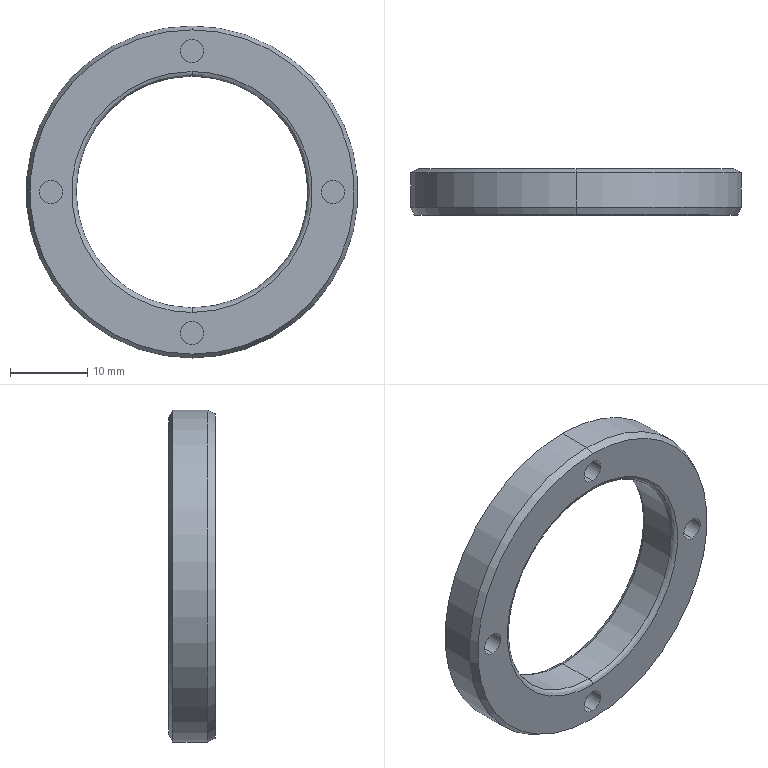Part | STEP file | _X2_8f9351fa95017d2773af_X0_MAB060_5.STEP.STEP | 1 solid | 31 faces | box 43 x 6 x 43 mm | volume 4269 mm3 | cylinder 12 | plane 11 | spline 4 | cone 4 | commonest cylinder face diameters 3 x8 30 x2 43 x2
STEP:
#1=CARTESIAN_POINT('',(0.,0.,15.6));
#2=VERTEX_POINT('',#1);
#3=CARTESIAN_POINT('',(0.,0.,-15.6));
#4=VERTEX_POINT('',#3);
#5=CARTESIAN_POINT('',(0.,0.,15.6));
#6=CARTESIAN_POINT('',(-31.2,0.,15.6));
#7=CARTESIAN_POINT('',(-31.2,0.,-15.6));
#8=CARTESIAN_POINT('',(0.,0.,-15.6));
#9=(BOUNDED_CURVE()B_SPLINE_CURVE(3,(#5,#6,#7,#8),.UNSPECIFIED.,.F.,.F.)B_SPLINE_CURVE_WITH_KNOTS((4,4),(0.,1.),.UNSPECIFIED.)CURVE()GEOMETRIC_REPRESENTATION_ITEM()RATIONAL_B_SPLINE_CURVE((1.,0.3333,0.3333,1.))REPRESENTATION_ITEM(''));
#10=EDGE_CURVE('',#2,#4,#9,.T.);
#11=ORIENTED_EDGE('',*,*,#10,.T.);
#12=CARTESIAN_POINT('',(0.,0.6,-15.));
#13=VERTEX_POINT('',#12);
#14=CARTESIAN_POINT('',(0.,0.6,-15.6));
#15=DIRECTION('',(-1.,0.,0.));
#16=DIRECTION('',(0.,0.,-1.));
#17=AXIS2_PLACEMENT_3D('',#14,#15,#16);
#18=CIRCLE('',#17,0.6);
#19=EDGE_CURVE('',#4,#13,#18,.T.);
#20=ORIENTED_EDGE('',*,*,#19,.T.);
#21=CARTESIAN_POINT('',(0.,0.6,15.));
#22=VERTEX_POINT('',#21);
#23=CARTESIAN_POINT('',(0.,0.6,0.));
#24=DIRECTION('',(0.,1.,0.));
#25=DIRECTION('',(0.,0.,1.));
#26=AXIS2_PLACEMENT_3D('',#23,#24,#25);
#27=CIRCLE('',#26,15.);
#28=EDGE_CURVE('',#13,#22,#27,.T.);
#29=ORIENTED_EDGE('',*,*,#28,.T.);
#30=CARTESIAN_POINT('',(0.,0.6,15.6));
#31=DIRECTION('',(1.,0.,0.));
#32=DIRECTION('',(0.,0.,1.));
#33=AXIS2_PLACEMENT_3D('',#30,#31,#32);
#34=CIRCLE('',#33,0.6);
#35=EDGE_CURVE('',#2,#22,#34,.T.);
#36=ORIENTED_EDGE('',*,*,#35,.F.);
#37=EDGE_LOOP('',(#11,#20,#29,#36));
#38=FACE_OUTER_BOUND('',#37,.T.);
#39=CARTESIAN_POINT('',(0.,0.,-15.6));
#40=CARTESIAN_POINT('',(-31.2,0.,-15.6));
#41=CARTESIAN_POINT('',(-31.2,0.,15.6));
#42=CARTESIAN_POINT('',(0.,0.,15.6));
#43=CARTESIAN_POINT('',(0.,0.,-15.249));
#44=CARTESIAN_POINT('',(-30.497,0.,-15.249));
#45=CARTESIAN_POINT('',(-30.497,0.,15.249));
#46=CARTESIAN_POINT('',(0.,0.,15.249));
#47=CARTESIAN_POINT('',(0.,0.2485,-15.));
#48=CARTESIAN_POINT('',(-30.,0.2485,-15.));
#49=CARTESIAN_POINT('',(-30.,0.2485,15.));
#50=CARTESIAN_POINT('',(0.,0.2485,15.));
#51=CARTESIAN_POINT('',(0.,0.6,-15.));
#52=CARTESIAN_POINT('',(-30.,0.6,-15.));
#53=CARTESIAN_POINT('',(-30.,0.6,15.));
#54=CARTESIAN_POINT('',(0.,0.6,15.));
#55=(BOUNDED_SURFACE()B_SPLINE_SURFACE(3,3,((#39,#40,#41,#42),(#43,#44,#45,#46),(#47,#48,#49,#50),(#51,#52,#53,#54)),.UNSPECIFIED.,.F.,.F.,.F.)B_SPLINE_SURFACE_WITH_KNOTS((4,4),(4,4),(0.,1.),(0.,1.),.UNSPECIFIED.)GEOMETRIC_REPRESENTATION_ITEM()RATIONAL_B_SPLINE_SURFACE(((1.,0.3333,0.3333,1.),(0.8047,0.2682,0.2682,0.8047),(0.8047,0.2682,0.2682,0.8047),(1.,0.3333,0.3333,1.)))REPRESENTATION_ITEM('')SURFACE());
#56=ADVANCED_FACE('',(#38),#55,.T.);
#57=CARTESIAN_POINT('',(0.,5.4,15.));
#58=VERTEX_POINT('',#57);
#59=CARTESIAN_POINT('',(0.,5.4,-15.));
#60=VERTEX_POINT('',#59);
#61=CARTESIAN_POINT('',(0.,5.4,0.));
#62=DIRECTION('',(0.,-1.,0.));
#63=DIRECTION('',(0.,0.,1.));
#64=AXIS2_PLACEMENT_3D('',#61,#62,#63);
#65=CIRCLE('',#64,15.);
#66=EDGE_CURVE('',#58,#60,#65,.T.);
#67=ORIENTED_EDGE('',*,*,#66,.T.);
#68=CARTESIAN_POINT('',(0.,6.,-15.6));
#69=VERTEX_POINT('',#68);
#70=CARTESIAN_POINT('',(0.,5.4,-15.6));
#71=DIRECTION('',(-1.,0.,0.));
#72=DIRECTION('',(0.,0.,-1.));
#73=AXIS2_PLACEMENT_3D('',#70,#71,#72);
#74=CIRCLE('',#73,0.6);
#75=EDGE_CURVE('',#60,#69,#74,.T.);
#76=ORIENTED_EDGE('',*,*,#75,.T.);
#77=CARTESIAN_POINT('',(0.,6.,15.6));
#78=VERTEX_POINT('',#77);
#79=CARTESIAN_POINT('',(0.,6.,-15.6));
#80=CARTESIAN_POINT('',(-31.2,6.,-15.6));
#81=CARTESIAN_POINT('',(-31.2,6.,15.6));
#82=CARTESIAN_POINT('',(0.,6.,15.6));
#83=(BOUNDED_CURVE()B_SPLINE_CURVE(3,(#79,#80,#81,#82),.UNSPECIFIED.,.F.,.F.)B_SPLINE_CURVE_WITH_KNOTS((4,4),(0.,1.),.UNSPECIFIED.)CURVE()GEOMETRIC_REPRESENTATION_ITEM()RATIONAL_B_SPLINE_CURVE((1.,0.3333,0.3333,1.))REPRESENTATION_ITEM(''));
#84=EDGE_CURVE('',#69,#78,#83,.T.);
#85=ORIENTED_EDGE('',*,*,#84,.T.);
#86=CARTESIAN_POINT('',(0.,5.4,15.6));
#87=DIRECTION('',(1.,0.,0.));
#88=DIRECTION('',(0.,0.,1.));
#89=AXIS2_PLACEMENT_3D('',#86,#87,#88);
#90=CIRCLE('',#89,0.6);
#91=EDGE_CURVE('',#58,#78,#90,.T.);
#92=ORIENTED_EDGE('',*,*,#91,.F.);
#93=EDGE_LOOP('',(#67,#76,#85,#92));
#94=FACE_OUTER_BOUND('',#93,.T.);
#95=CARTESIAN_POINT('',(0.,5.4,-15.));
#96=CARTESIAN_POINT('',(-30.,5.4,-15.));
#97=CARTESIAN_POINT('',(-30.,5.4,15.));
#98=CARTESIAN_POINT('',(0.,5.4,15.));
#99=CARTESIAN_POINT('',(0.,5.751,-15.));
#100=CARTESIAN_POINT('',(-30.,5.751,-15.));
#101=CARTESIAN_POINT('',(-30.,5.751,15.));
#102=CARTESIAN_POINT('',(0.,5.751,15.));
#103=CARTESIAN_POINT('',(0.,6.,-15.249));
#104=CARTESIAN_POINT('',(-30.497,6.,-15.249));
#105=CARTESIAN_POINT('',(-30.497,6.,15.249));
#106=CARTESIAN_POINT('',(0.,6.,15.249));
#107=CARTESIAN_POINT('',(0.,6.,-15.6));
#108=CARTESIAN_POINT('',(-31.2,6.,-15.6));
#109=CARTESIAN_POINT('',(-31.2,6.,15.6));
#110=CARTESIAN_POINT('',(0.,6.,15.6));
#111=(BOUNDED_SURFACE()B_SPLINE_SURFACE(3,3,((#95,#96,#97,#98),(#99,#100,#101,#102),(#103,#104,#105,#106),(#107,#108,#109,#110)),.UNSPECIFIED.,.F.,.F.,.F.)B_SPLINE_SURFACE_WITH_KNOTS((4,4),(4,4),(0.,1.),(0.,1.),.UNSPECIFIED.)GEOMETRIC_REPRESENTATION_ITEM()RATIONAL_B_SPLINE_SURFACE(((1.,0.3333,0.3333,1.),(0.8047,0.2682,0.2682,0.8047),(0.8047,0.2682,0.2682,0.8047),(1.,0.3333,0.3333,1.)))REPRESENTATION_ITEM('')SURFACE());
#112=ADVANCED_FACE('',(#94),#111,.T.);
#113=CARTESIAN_POINT('',(0.,0.,21.));
#114=VERTEX_POINT('',#113);
#115=CARTESIAN_POINT('',(0.,0.,-21.));
#116=VERTEX_POINT('',#115);
#117=CARTESIAN_POINT('',(0.,0.,0.));
#118=DIRECTION('',(0.,1.,0.));
#119=DIRECTION('',(0.,0.,1.));
#120=AXIS2_PLACEMENT_3D('',#117,#118,#119);
#121=CIRCLE('',#120,21.);
#122=EDGE_CURVE('',#114,#116,#121,.T.);
#123=ORIENTED_EDGE('',*,*,#122,.T.);
#124=CARTESIAN_POINT('',(0.,1.,-21.5));
#125=VERTEX_POINT('',#124);
#126=CARTESIAN_POINT('',(0.,1.,-21.5));
#127=DIRECTION('',(0.,0.8944,-0.4472));
#128=VECTOR('',#127,1000.);
#129=LINE('',#126,#128);
#130=EDGE_CURVE('',#116,#125,#129,.T.);
#131=ORIENTED_EDGE('',*,*,#130,.T.);
#132=CARTESIAN_POINT('',(0.,1.,21.5));
#133=VERTEX_POINT('',#132);
#134=CARTESIAN_POINT('',(0.,1.,0.));
#135=DIRECTION('',(0.,-1.,0.));
#136=DIRECTION('',(0.,0.,1.));
#137=AXIS2_PLACEMENT_3D('',#134,#135,#136);
#138=CIRCLE('',#137,21.5);
#139=EDGE_CURVE('',#125,#133,#138,.T.);
#140=ORIENTED_EDGE('',*,*,#139,.T.);
#141=CARTESIAN_POINT('',(0.,1.,21.5));
#142=DIRECTION('',(0.,0.8944,0.4472));
#143=VECTOR('',#142,1000.);
#144=LINE('',#141,#143);
#145=EDGE_CURVE('',#114,#133,#144,.T.);
#146=ORIENTED_EDGE('',*,*,#145,.F.);
#147=EDGE_LOOP('',(#123,#131,#140,#146));
#148=FACE_OUTER_BOUND('',#147,.T.);
#149=CARTESIAN_POINT('',(0.,1.,0.));
#150=DIRECTION('',(0.,1.,0.));
#151=DIRECTION('',(0.,0.,1.));
#152=AXIS2_PLACEMENT_3D('',#149,#150,#151);
#153=CONICAL_SURFACE('',#152,21.5,0.4636);
#154=ADVANCED_FACE('',(#148),#153,.T.);
#155=CARTESIAN_POINT('',(0.,4.,-16.75));
#156=VERTEX_POINT('',#155);
#157=CARTESIAN_POINT('',(0.,4.,-19.75));
#158=VERTEX_POINT('',#157);
#159=CARTESIAN_POINT('',(0.,4.,-18.25));
#160=DIRECTION('',(0.,-1.,0.));
#161=DIRECTION('',(0.,0.,-1.));
#162=AXIS2_PLACEMENT_3D('',#159,#160,#161);
#163=CIRCLE('',#162,1.5);
#164=EDGE_CURVE('',#156,#158,#163,.T.);
#165=ORIENTED_EDGE('',*,*,#164,.F.);
#166=CARTESIAN_POINT('',(0.,0.,-16.75));
#167=VERTEX_POINT('',#166);
#168=CARTESIAN_POINT('',(0.,4.,-16.75));
#169=DIRECTION('',(0.,-1.,0.));
#170=VECTOR('',#169,1000.);
#171=LINE('',#168,#170);
#172=EDGE_CURVE('',#156,#167,#171,.T.);
#173=ORIENTED_EDGE('',*,*,#172,.T.);
#174=CARTESIAN_POINT('',(0.,0.,-19.75));
#175=VERTEX_POINT('',#174);
#176=CARTESIAN_POINT('',(0.,0.,-18.25));
#177=DIRECTION('',(0.,-1.,0.));
#178=DIRECTION('',(0.,0.,-1.));
#179=AXIS2_PLACEMENT_3D('',#176,#177,#178);
#180=CIRCLE('',#179,1.5);
#181=EDGE_CURVE('',#167,#175,#180,.T.);
#182=ORIENTED_EDGE('',*,*,#181,.T.);
#183=CARTESIAN_POINT('',(0.,4.,-19.75));
#184=DIRECTION('',(0.,-1.,0.));
#185=VECTOR('',#184,1000.);
#186=LINE('',#183,#185);
#187=EDGE_CURVE('',#158,#175,#186,.T.);
#188=ORIENTED_EDGE('',*,*,#187,.F.);
#189=EDGE_LOOP('',(#165,#173,#182,#188));
#190=FACE_OUTER_BOUND('',#189,.T.);
#191=CARTESIAN_POINT('',(0.,4.,-18.25));
#192=DIRECTION('',(0.,-1.,0.));
#193=DIRECTION('',(0.,0.,-1.));
#194=AXIS2_PLACEMENT_3D('',#191,#192,#193);
#195=CYLINDRICAL_SURFACE('',#194,1.5);
#196=ADVANCED_FACE('',(#190),#195,.F.);
#197=CARTESIAN_POINT('',(-18.25,4.,1.5));
#198=VERTEX_POINT('',#197);
#199=CARTESIAN_POINT('',(-18.25,4.,-1.5));
#200=VERTEX_POINT('',#199);
#201=CARTESIAN_POINT('',(-18.25,4.,0.));
#202=DIRECTION('',(0.,-1.,0.));
#203=DIRECTION('',(0.,0.,-1.));
#204=AXIS2_PLACEMENT_3D('',#201,#202,#203);
#205=CIRCLE('',#204,1.5);
#206=EDGE_CURVE('',#198,#200,#205,.T.);
#207=ORIENTED_EDGE('',*,*,#206,.F.);
#208=CARTESIAN_POINT('',(-18.25,0.,1.5));
#209=VERTEX_POINT('',#208);
#210=CARTESIAN_POINT('',(-18.25,4.,1.5));
#211=DIRECTION('',(0.,-1.,0.));
#212=VECTOR('',#211,1000.);
#213=LINE('',#210,#212);
#214=EDGE_CURVE('',#198,#209,#213,.T.);
#215=ORIENTED_EDGE('',*,*,#214,.T.);
#216=CARTESIAN_POINT('',(-18.25,0.,-1.5));
#217=VERTEX_POINT('',#216);
#218=CARTESIAN_POINT('',(-18.25,0.,0.));
#219=DIRECTION('',(0.,-1.,0.));
#220=DIRECTION('',(0.,0.,-1.));
#221=AXIS2_PLACEMENT_3D('',#218,#219,#220);
#222=CIRCLE('',#221,1.5);
#223=EDGE_CURVE('',#209,#217,#222,.T.);
#224=ORIENTED_EDGE('',*,*,#223,.T.);
#225=CARTESIAN_POINT('',(-18.25,4.,-1.5));
#226=DIRECTION('',(0.,-1.,0.));
#227=VECTOR('',#226,1000.);
#228=LINE('',#225,#227);
#229=EDGE_CURVE('',#200,#217,#228,.T.);
#230=ORIENTED_EDGE('',*,*,#229,.F.);
#231=EDGE_LOOP('',(#207,#215,#224,#230));
#232=FACE_OUTER_BOUND('',#231,.T.);
#233=CARTESIAN_POINT('',(-18.25,4.,0.));
#234=DIRECTION('',(0.,-1.,0.));
#235=DIRECTION('',(0.,0.,-1.));
#236=AXIS2_PLACEMENT_3D('',#233,#234,#235);
#237=CYLINDRICAL_SURFACE('',#236,1.5);
#238=ADVANCED_FACE('',(#232),#237,.F.);
#239=CARTESIAN_POINT('',(0.,4.,19.75));
#240=VERTEX_POINT('',#239);
#241=CARTESIAN_POINT('',(0.,4.,16.75));
#242=VERTEX_POINT('',#241);
#243=CARTESIAN_POINT('',(0.,4.,18.25));
#244=DIRECTION('',(0.,-1.,0.));
#245=DIRECTION('',(0.,0.,-1.));
#246=AXIS2_PLACEMENT_3D('',#243,#244,#245);
#247=CIRCLE('',#246,1.5);
#248=EDGE_CURVE('',#240,#242,#247,.T.);
#249=ORIENTED_EDGE('',*,*,#248,.F.);
#250=CARTESIAN_POINT('',(0.,0.,19.75));
#251=VERTEX_POINT('',#250);
#252=CARTESIAN_POINT('',(0.,4.,19.75));
#253=DIRECTION('',(0.,-1.,0.));
#254=VECTOR('',#253,1000.);
#255=LINE('',#252,#254);
#256=EDGE_CURVE('',#240,#251,#255,.T.);
#257=ORIENTED_EDGE('',*,*,#256,.T.);
#258=CARTESIAN_POINT('',(0.,0.,16.75));
#259=VERTEX_POINT('',#258);
#260=CARTESIAN_POINT('',(0.,0.,18.25));
#261=DIRECTION('',(0.,-1.,0.));
#262=DIRECTION('',(0.,0.,-1.));
#263=AXIS2_PLACEMENT_3D('',#260,#261,#262);
#264=CIRCLE('',#263,1.5);
#265=EDGE_CURVE('',#251,#259,#264,.T.);
#266=ORIENTED_EDGE('',*,*,#265,.T.);
#267=CARTESIAN_POINT('',(0.,4.,16.75));
#268=DIRECTION('',(0.,-1.,0.));
#269=VECTOR('',#268,1000.);
#270=LINE('',#267,#269);
#271=EDGE_CURVE('',#242,#259,#270,.T.);
#272=ORIENTED_EDGE('',*,*,#271,.F.);
#273=EDGE_LOOP('',(#249,#257,#266,#272));
#274=FACE_OUTER_BOUND('',#273,.T.);
#275=CARTESIAN_POINT('',(0.,4.,18.25));
#276=DIRECTION('',(0.,-1.,0.));
#277=DIRECTION('',(0.,0.,-1.));
#278=AXIS2_PLACEMENT_3D('',#275,#276,#277);
#279=CYLINDRICAL_SURFACE('',#278,1.5);
#280=ADVANCED_FACE('',(#274),#279,.F.);
#281=CARTESIAN_POINT('',(18.25,4.,1.5));
#282=VERTEX_POINT('',#281);
#283=CARTESIAN_POINT('',(18.25,4.,-1.5));
#284=VERTEX_POINT('',#283);
#285=CARTESIAN_POINT('',(18.25,4.,0.));
#286=DIRECTION('',(0.,-1.,0.));
#287=DIRECTION('',(0.,0.,-1.));
#288=AXIS2_PLACEMENT_3D('',#285,#286,#287);
#289=CIRCLE('',#288,1.5);
#290=EDGE_CURVE('',#282,#284,#289,.T.);
#291=ORIENTED_EDGE('',*,*,#290,.F.);
#292=CARTESIAN_POINT('',(18.25,0.,1.5));
#293=VERTEX_POINT('',#292);
#294=CARTESIAN_POINT('',(18.25,4.,1.5));
#295=DIRECTION('',(0.,-1.,0.));
#296=VECTOR('',#295,1000.);
#297=LINE('',#294,#296);
#298=EDGE_CURVE('',#282,#293,#297,.T.);
#299=ORIENTED_EDGE('',*,*,#298,.T.);
#300=CARTESIAN_POINT('',(18.25,0.,-1.5));
#301=VERTEX_POINT('',#300);
#302=CARTESIAN_POINT('',(18.25,0.,0.));
#303=DIRECTION('',(0.,-1.,0.));
#304=DIRECTION('',(0.,0.,-1.));
#305=AXIS2_PLACEMENT_3D('',#302,#303,#304);
#306=CIRCLE('',#305,1.5);
#307=EDGE_CURVE('',#293,#301,#306,.T.);
#308=ORIENTED_EDGE('',*,*,#307,.T.);
#309=CARTESIAN_POINT('',(18.25,4.,-1.5));
#310=DIRECTION('',(0.,-1.,0.));
#311=VECTOR('',#310,1000.);
#312=LINE('',#309,#311);
#313=EDGE_CURVE('',#284,#301,#312,.T.);
#314=ORIENTED_EDGE('',*,*,#313,.F.);
#315=EDGE_LOOP('',(#291,#299,#308,#314));
#316=FACE_OUTER_BOUND('',#315,.T.);
#317=CARTESIAN_POINT('',(18.25,4.,0.));
#318=DIRECTION('',(0.,-1.,0.));
#319=DIRECTION('',(0.,0.,-1.));
#320=AXIS2_PLACEMENT_3D('',#317,#318,#319);
#321=CYLINDRICAL_SURFACE('',#320,1.5);
#322=ADVANCED_FACE('',(#316),#321,.F.);
#323=CARTESIAN_POINT('',(0.,5.5,-21.5));
#324=VERTEX_POINT('',#323);
#325=CARTESIAN_POINT('',(0.,5.5,21.5));
#326=VERTEX_POINT('',#325);
#327=CARTESIAN_POINT('',(0.,5.5,0.));
#328=DIRECTION('',(0.,-1.,0.));
#329=DIRECTION('',(0.,0.,-1.));
#330=AXIS2_PLACEMENT_3D('',#327,#328,#329);
#331=CIRCLE('',#330,21.5);
#332=EDGE_CURVE('',#324,#326,#331,.T.);
#333=ORIENTED_EDGE('',*,*,#332,.T.);
#334=CARTESIAN_POINT('',(0.,6.,21.5));
#335=DIRECTION('',(0.,-1.,0.));
#336=VECTOR('',#335,1000.);
#337=LINE('',#334,#336);
#338=EDGE_CURVE('',#326,#133,#337,.T.);
#339=ORIENTED_EDGE('',*,*,#338,.T.);
#340=ORIENTED_EDGE('',*,*,#139,.F.);
#341=CARTESIAN_POINT('',(0.,6.,-21.5));
#342=DIRECTION('',(0.,-1.,0.));
#343=VECTOR('',#342,1000.);
#344=LINE('',#341,#343);
#345=EDGE_CURVE('',#324,#125,#344,.T.);
#346=ORIENTED_EDGE('',*,*,#345,.F.);
#347=EDGE_LOOP('',(#333,#339,#340,#346));
#348=FACE_OUTER_BOUND('',#347,.T.);
#349=CARTESIAN_POINT('',(0.,6.,0.));
#350=DIRECTION('',(0.,-1.,0.));
#351=DIRECTION('',(0.,0.,-1.));
#352=AXIS2_PLACEMENT_3D('',#349,#350,#351);
#353=CYLINDRICAL_SURFACE('',#352,21.5);
#354=ADVANCED_FACE('',(#348),#353,.T.);
#355=ORIENTED_EDGE('',*,*,#28,.F.);
#356=CARTESIAN_POINT('',(0.,0.,-15.));
#357=DIRECTION('',(0.,1.,0.));
#358=VECTOR('',#357,1000.);
#359=LINE('',#356,#358);
#360=EDGE_CURVE('',#13,#60,#359,.T.);
#361=ORIENTED_EDGE('',*,*,#360,.T.);
#362=ORIENTED_EDGE('',*,*,#66,.F.);
#363=CARTESIAN_POINT('',(0.,0.,15.));
#364=DIRECTION('',(0.,1.,0.));
#365=VECTOR('',#364,1000.);
#366=LINE('',#363,#365);
#367=EDGE_CURVE('',#22,#58,#366,.T.);
#368=ORIENTED_EDGE('',*,*,#367,.F.);
#369=EDGE_LOOP('',(#355,#361,#362,#368));
#370=FACE_OUTER_BOUND('',#369,.T.);
#371=CARTESIAN_POINT('',(0.,0.,0.));
#372=DIRECTION('',(0.,1.,0.));
#373=DIRECTION('',(0.,0.,1.));
#374=AXIS2_PLACEMENT_3D('',#371,#372,#373);
#375=CYLINDRICAL_SURFACE('',#374,15.);
#376=ADVANCED_FACE('',(#370),#375,.F.);
#377=CARTESIAN_POINT('',(0.,6.,-20.5));
#378=VERTEX_POINT('',#377);
#379=CARTESIAN_POINT('',(0.,6.,20.5));
#380=VERTEX_POINT('',#379);
#381=CARTESIAN_POINT('',(0.,6.,0.));
#382=DIRECTION('',(0.,-1.,0.));
#383=DIRECTION('',(0.,0.,-1.));
#384=AXIS2_PLACEMENT_3D('',#381,#382,#383);
#385=CIRCLE('',#384,20.5);
#386=EDGE_CURVE('',#378,#380,#385,.T.);
#387=ORIENTED_EDGE('',*,*,#386,.T.);
#388=CARTESIAN_POINT('',(0.,5.5,21.5));
#389=DIRECTION('',(0.,-0.4472,0.8944));
#390=VECTOR('',#389,1000.);
#391=LINE('',#388,#390);
#392=EDGE_CURVE('',#380,#326,#391,.T.);
#393=ORIENTED_EDGE('',*,*,#392,.T.);
#394=ORIENTED_EDGE('',*,*,#332,.F.);
#395=CARTESIAN_POINT('',(0.,5.5,-21.5));
#396=DIRECTION('',(0.,-0.4472,-0.8944));
#397=VECTOR('',#396,1000.);
#398=LINE('',#395,#397);
#399=EDGE_CURVE('',#378,#324,#398,.T.);
#400=ORIENTED_EDGE('',*,*,#399,.F.);
#401=EDGE_LOOP('',(#387,#393,#394,#400));
#402=FACE_OUTER_BOUND('',#401,.T.);
#403=CARTESIAN_POINT('',(0.,5.5,0.));
#404=DIRECTION('',(0.,-1.,0.));
#405=DIRECTION('',(0.,0.,-1.));
#406=AXIS2_PLACEMENT_3D('',#403,#404,#405);
#407=CONICAL_SURFACE('',#406,21.5,1.107);
#408=ADVANCED_FACE('',(#402),#407,.T.);
#409=ORIENTED_EDGE('',*,*,#122,.F.);
#410=CARTESIAN_POINT('',(0.,0.,0.));
#411=DIRECTION('',(0.,1.,0.));
#412=DIRECTION('',(0.,0.,1.));
#413=AXIS2_PLACEMENT_3D('',#410,#411,#412);
#414=CIRCLE('',#413,21.);
#415=EDGE_CURVE('',#116,#114,#414,.T.);
#416=ORIENTED_EDGE('',*,*,#415,.F.);
#417=EDGE_LOOP('',(#409,#416));
#418=FACE_OUTER_BOUND('',#417,.T.);
#419=ORIENTED_EDGE('',*,*,#10,.F.);
#420=CARTESIAN_POINT('',(0.,0.,-15.6));
#421=CARTESIAN_POINT('',(31.2,0.,-15.6));
#422=CARTESIAN_POINT('',(31.2,0.,15.6));
#423=CARTESIAN_POINT('',(0.,0.,15.6));
#424=(BOUNDED_CURVE()B_SPLINE_CURVE(3,(#420,#421,#422,#423),.UNSPECIFIED.,.F.,.F.)B_SPLINE_CURVE_WITH_KNOTS((4,4),(0.,1.),.UNSPECIFIED.)CURVE()GEOMETRIC_REPRESENTATION_ITEM()RATIONAL_B_SPLINE_CURVE((1.,0.3333,0.3333,1.))REPRESENTATION_ITEM(''));
#425=EDGE_CURVE('',#4,#2,#424,.T.);
#426=ORIENTED_EDGE('',*,*,#425,.F.);
#427=EDGE_LOOP('',(#419,#426));
#428=FACE_BOUND('',#427,.T.);
#429=CARTESIAN_POINT('',(0.,0.,-18.25));
#430=DIRECTION('',(0.,-1.,0.));
#431=DIRECTION('',(0.,0.,-1.));
#432=AXIS2_PLACEMENT_3D('',#429,#430,#431);
#433=CIRCLE('',#432,1.5);
#434=EDGE_CURVE('',#175,#167,#433,.T.);
#435=ORIENTED_EDGE('',*,*,#434,.F.);
#436=ORIENTED_EDGE('',*,*,#181,.F.);
#437=EDGE_LOOP('',(#435,#436));
#438=FACE_BOUND('',#437,.T.);
#439=CARTESIAN_POINT('',(-18.25,0.,0.));
#440=DIRECTION('',(0.,-1.,0.));
#441=DIRECTION('',(0.,0.,-1.));
#442=AXIS2_PLACEMENT_3D('',#439,#440,#441);
#443=CIRCLE('',#442,1.5);
#444=EDGE_CURVE('',#217,#209,#443,.T.);
#445=ORIENTED_EDGE('',*,*,#444,.F.);
#446=ORIENTED_EDGE('',*,*,#223,.F.);
#447=EDGE_LOOP('',(#445,#446));
#448=FACE_BOUND('',#447,.T.);
#449=CARTESIAN_POINT('',(0.,0.,18.25));
#450=DIRECTION('',(0.,-1.,0.));
#451=DIRECTION('',(0.,0.,-1.));
#452=AXIS2_PLACEMENT_3D('',#449,#450,#451);
#453=CIRCLE('',#452,1.5);
#454=EDGE_CURVE('',#259,#251,#453,.T.);
#455=ORIENTED_EDGE('',*,*,#454,.F.);
#456=ORIENTED_EDGE('',*,*,#265,.F.);
#457=EDGE_LOOP('',(#455,#456));
#458=FACE_BOUND('',#457,.T.);
#459=CARTESIAN_POINT('',(18.25,0.,0.));
#460=DIRECTION('',(0.,-1.,0.));
#461=DIRECTION('',(0.,0.,-1.));
#462=AXIS2_PLACEMENT_3D('',#459,#460,#461);
#463=CIRCLE('',#462,1.5);
#464=EDGE_CURVE('',#301,#293,#463,.T.);
#465=ORIENTED_EDGE('',*,*,#464,.F.);
#466=ORIENTED_EDGE('',*,*,#307,.F.);
#467=EDGE_LOOP('',(#465,#466));
#468=FACE_BOUND('',#467,.T.);
#469=CARTESIAN_POINT('',(0.,0.,0.));
#470=DIRECTION('',(0.,1.,0.));
#471=DIRECTION('',(0.,0.,1.));
#472=AXIS2_PLACEMENT_3D('',#469,#470,#471);
#473=PLANE('',#472);
#474=ADVANCED_FACE('',(#418,#428,#438,#448,#458,#468),#473,.F.);
#475=ORIENTED_EDGE('',*,*,#130,.F.);
#476=ORIENTED_EDGE('',*,*,#415,.T.);
#477=ORIENTED_EDGE('',*,*,#145,.T.);
#478=CARTESIAN_POINT('',(0.,1.,0.));
#479=DIRECTION('',(0.,-1.,0.));
#480=DIRECTION('',(0.,0.,1.));
#481=AXIS2_PLACEMENT_3D('',#478,#479,#480);
#482=CIRCLE('',#481,21.5);
#483=EDGE_CURVE('',#133,#125,#482,.T.);
#484=ORIENTED_EDGE('',*,*,#483,.T.);
#485=EDGE_LOOP('',(#475,#476,#477,#484));
#486=FACE_OUTER_BOUND('',#485,.T.);
#487=CARTESIAN_POINT('',(0.,1.,0.));
#488=DIRECTION('',(0.,1.,0.));
#489=DIRECTION('',(0.,0.,1.));
#490=AXIS2_PLACEMENT_3D('',#487,#488,#489);
#491=CONICAL_SURFACE('',#490,21.5,0.4636);
#492=ADVANCED_FACE('',(#486),#491,.T.);
#493=ORIENTED_EDGE('',*,*,#19,.F.);
#494=ORIENTED_EDGE('',*,*,#425,.T.);
#495=ORIENTED_EDGE('',*,*,#35,.T.);
#496=CARTESIAN_POINT('',(0.,0.6,0.));
#497=DIRECTION('',(0.,1.,0.));
#498=DIRECTION('',(0.,0.,1.));
#499=AXIS2_PLACEMENT_3D('',#496,#497,#498);
#500=CIRCLE('',#499,15.);
#501=EDGE_CURVE('',#22,#13,#500,.T.);
#502=ORIENTED_EDGE('',*,*,#501,.T.);
#503=EDGE_LOOP('',(#493,#494,#495,#502));
#504=FACE_OUTER_BOUND('',#503,.T.);
#505=CARTESIAN_POINT('',(0.,0.,15.6));
#506=CARTESIAN_POINT('',(31.2,0.,15.6));
#507=CARTESIAN_POINT('',(31.2,0.,-15.6));
#508=CARTESIAN_POINT('',(0.,0.,-15.6));
#509=CARTESIAN_POINT('',(0.,0.,15.249));
#510=CARTESIAN_POINT('',(30.497,0.,15.249));
#511=CARTESIAN_POINT('',(30.497,0.,-15.249));
#512=CARTESIAN_POINT('',(0.,0.,-15.249));
#513=CARTESIAN_POINT('',(0.,0.2485,15.));
#514=CARTESIAN_POINT('',(30.,0.2485,15.));
#515=CARTESIAN_POINT('',(30.,0.2485,-15.));
#516=CARTESIAN_POINT('',(0.,0.2485,-15.));
#517=CARTESIAN_POINT('',(0.,0.6,15.));
#518=CARTESIAN_POINT('',(30.,0.6,15.));
#519=CARTESIAN_POINT('',(30.,0.6,-15.));
#520=CARTESIAN_POINT('',(0.,0.6,-15.));
#521=(BOUNDED_SURFACE()B_SPLINE_SURFACE(3,3,((#505,#506,#507,#508),(#509,#510,#511,#512),(#513,#514,#515,#516),(#517,#518,#519,#520)),.UNSPECIFIED.,.F.,.F.,.F.)B_SPLINE_SURFACE_WITH_KNOTS((4,4),(4,4),(0.,1.),(0.,1.),.UNSPECIFIED.)GEOMETRIC_REPRESENTATION_ITEM()RATIONAL_B_SPLINE_SURFACE(((1.,0.3333,0.3333,1.),(0.8047,0.2682,0.2682,0.8047),(0.8047,0.2682,0.2682,0.8047),(1.,0.3333,0.3333,1.)))REPRESENTATION_ITEM('')SURFACE());
#522=ADVANCED_FACE('',(#504),#521,.T.);
#523=ORIENTED_EDGE('',*,*,#172,.F.);
#524=CARTESIAN_POINT('',(0.,4.,-18.25));
#525=DIRECTION('',(0.,-1.,0.));
#526=DIRECTION('',(0.,0.,-1.));
#527=AXIS2_PLACEMENT_3D('',#524,#525,#526);
#528=CIRCLE('',#527,1.5);
#529=EDGE_CURVE('',#158,#156,#528,.T.);
#530=ORIENTED_EDGE('',*,*,#529,.F.);
#531=ORIENTED_EDGE('',*,*,#187,.T.);
#532=ORIENTED_EDGE('',*,*,#434,.T.);
#533=EDGE_LOOP('',(#523,#530,#531,#532));
#534=FACE_OUTER_BOUND('',#533,.T.);
#535=CARTESIAN_POINT('',(0.,4.,-18.25));
#536=DIRECTION('',(0.,-1.,0.));
#537=DIRECTION('',(0.,0.,-1.));
#538=AXIS2_PLACEMENT_3D('',#535,#536,#537);
#539=CYLINDRICAL_SURFACE('',#538,1.5);
#540=ADVANCED_FACE('',(#534),#539,.F.);
#541=ORIENTED_EDGE('',*,*,#214,.F.);
#542=CARTESIAN_POINT('',(-18.25,4.,0.));
#543=DIRECTION('',(0.,-1.,0.));
#544=DIRECTION('',(0.,0.,-1.));
#545=AXIS2_PLACEMENT_3D('',#542,#543,#544);
#546=CIRCLE('',#545,1.5);
#547=EDGE_CURVE('',#200,#198,#546,.T.);
#548=ORIENTED_EDGE('',*,*,#547,.F.);
#549=ORIENTED_EDGE('',*,*,#229,.T.);
#550=ORIENTED_EDGE('',*,*,#444,.T.);
#551=EDGE_LOOP('',(#541,#548,#549,#550));
#552=FACE_OUTER_BOUND('',#551,.T.);
#553=CARTESIAN_POINT('',(-18.25,4.,0.));
#554=DIRECTION('',(0.,-1.,0.));
#555=DIRECTION('',(0.,0.,-1.));
#556=AXIS2_PLACEMENT_3D('',#553,#554,#555);
#557=CYLINDRICAL_SURFACE('',#556,1.5);
#558=ADVANCED_FACE('',(#552),#557,.F.);
#559=ORIENTED_EDGE('',*,*,#256,.F.);
#560=CARTESIAN_POINT('',(0.,4.,18.25));
#561=DIRECTION('',(0.,-1.,0.));
#562=DIRECTION('',(0.,0.,-1.));
#563=AXIS2_PLACEMENT_3D('',#560,#561,#562);
#564=CIRCLE('',#563,1.5);
#565=EDGE_CURVE('',#242,#240,#564,.T.);
#566=ORIENTED_EDGE('',*,*,#565,.F.);
#567=ORIENTED_EDGE('',*,*,#271,.T.);
#568=ORIENTED_EDGE('',*,*,#454,.T.);
#569=EDGE_LOOP('',(#559,#566,#567,#568));
#570=FACE_OUTER_BOUND('',#569,.T.);
#571=CARTESIAN_POINT('',(0.,4.,18.25));
#572=DIRECTION('',(0.,-1.,0.));
#573=DIRECTION('',(0.,0.,-1.));
#574=AXIS2_PLACEMENT_3D('',#571,#572,#573);
#575=CYLINDRICAL_SURFACE('',#574,1.5);
#576=ADVANCED_FACE('',(#570),#575,.F.);
#577=ORIENTED_EDGE('',*,*,#298,.F.);
#578=CARTESIAN_POINT('',(18.25,4.,0.));
#579=DIRECTION('',(0.,-1.,0.));
#580=DIRECTION('',(0.,0.,-1.));
#581=AXIS2_PLACEMENT_3D('',#578,#579,#580);
#582=CIRCLE('',#581,1.5);
#583=EDGE_CURVE('',#284,#282,#582,.T.);
#584=ORIENTED_EDGE('',*,*,#583,.F.);
#585=ORIENTED_EDGE('',*,*,#313,.T.);
#586=ORIENTED_EDGE('',*,*,#464,.T.);
#587=EDGE_LOOP('',(#577,#584,#585,#586));
#588=FACE_OUTER_BOUND('',#587,.T.);
#589=CARTESIAN_POINT('',(18.25,4.,0.));
#590=DIRECTION('',(0.,-1.,0.));
#591=DIRECTION('',(0.,0.,-1.));
#592=AXIS2_PLACEMENT_3D('',#589,#590,#591);
#593=CYLINDRICAL_SURFACE('',#592,1.5);
#594=ADVANCED_FACE('',(#588),#593,.F.);
#595=ORIENTED_EDGE('',*,*,#338,.F.);
#596=CARTESIAN_POINT('',(0.,5.5,0.));
#597=DIRECTION('',(0.,-1.,0.));
#598=DIRECTION('',(0.,0.,-1.));
#599=AXIS2_PLACEMENT_3D('',#596,#597,#598);
#600=CIRCLE('',#599,21.5);
#601=EDGE_CURVE('',#326,#324,#600,.T.);
#602=ORIENTED_EDGE('',*,*,#601,.T.);
#603=ORIENTED_EDGE('',*,*,#345,.T.);
#604=ORIENTED_EDGE('',*,*,#483,.F.);
#605=EDGE_LOOP('',(#595,#602,#603,#604));
#606=FACE_OUTER_BOUND('',#605,.T.);
#607=CARTESIAN_POINT('',(0.,6.,0.));
#608=DIRECTION('',(0.,-1.,0.));
#609=DIRECTION('',(0.,0.,-1.));
#610=AXIS2_PLACEMENT_3D('',#607,#608,#609);
#611=CYLINDRICAL_SURFACE('',#610,21.5);
#612=ADVANCED_FACE('',(#606),#611,.T.);
#613=ORIENTED_EDGE('',*,*,#360,.F.);
#614=ORIENTED_EDGE('',*,*,#501,.F.);
#615=ORIENTED_EDGE('',*,*,#367,.T.);
#616=CARTESIAN_POINT('',(0.,5.4,0.));
#617=DIRECTION('',(0.,-1.,0.));
#618=DIRECTION('',(0.,0.,1.));
#619=AXIS2_PLACEMENT_3D('',#616,#617,#618);
#620=CIRCLE('',#619,15.);
#621=EDGE_CURVE('',#60,#58,#620,.T.);
#622=ORIENTED_EDGE('',*,*,#621,.F.);
#623=EDGE_LOOP('',(#613,#614,#615,#622));
#624=FACE_OUTER_BOUND('',#623,.T.);
#625=CARTESIAN_POINT('',(0.,0.,0.));
#626=DIRECTION('',(0.,1.,0.));
#627=DIRECTION('',(0.,0.,1.));
#628=AXIS2_PLACEMENT_3D('',#625,#626,#627);
#629=CYLINDRICAL_SURFACE('',#628,15.);
#630=ADVANCED_FACE('',(#624),#629,.F.);
#631=ORIENTED_EDGE('',*,*,#529,.T.);
#632=ORIENTED_EDGE('',*,*,#164,.T.);
#633=EDGE_LOOP('',(#631,#632));
#634=FACE_OUTER_BOUND('',#633,.T.);
#635=CARTESIAN_POINT('',(0.,4.,-18.25));
#636=DIRECTION('',(0.,1.,0.));
#637=DIRECTION('',(0.,0.,1.));
#638=AXIS2_PLACEMENT_3D('',#635,#636,#637);
#639=PLANE('',#638);
#640=ADVANCED_FACE('',(#634),#639,.F.);
#641=ORIENTED_EDGE('',*,*,#547,.T.);
#642=ORIENTED_EDGE('',*,*,#206,.T.);
#643=EDGE_LOOP('',(#641,#642));
#644=FACE_OUTER_BOUND('',#643,.T.);
#645=CARTESIAN_POINT('',(-18.25,4.,0.));
#646=DIRECTION('',(0.,1.,0.));
#647=DIRECTION('',(0.,0.,1.));
#648=AXIS2_PLACEMENT_3D('',#645,#646,#647);
#649=PLANE('',#648);
#650=ADVANCED_FACE('',(#644),#649,.F.);
#651=ORIENTED_EDGE('',*,*,#565,.T.);
#652=ORIENTED_EDGE('',*,*,#248,.T.);
#653=EDGE_LOOP('',(#651,#652));
#654=FACE_OUTER_BOUND('',#653,.T.);
#655=CARTESIAN_POINT('',(0.,4.,18.25));
#656=DIRECTION('',(0.,1.,0.));
#657=DIRECTION('',(0.,0.,1.));
#658=AXIS2_PLACEMENT_3D('',#655,#656,#657);
#659=PLANE('',#658);
#660=ADVANCED_FACE('',(#654),#659,.F.);
#661=ORIENTED_EDGE('',*,*,#583,.T.);
#662=ORIENTED_EDGE('',*,*,#290,.T.);
#663=EDGE_LOOP('',(#661,#662));
#664=FACE_OUTER_BOUND('',#663,.T.);
#665=CARTESIAN_POINT('',(18.25,4.,0.));
#666=DIRECTION('',(0.,1.,0.));
#667=DIRECTION('',(0.,0.,1.));
#668=AXIS2_PLACEMENT_3D('',#665,#666,#667);
#669=PLANE('',#668);
#670=ADVANCED_FACE('',(#664),#669,.F.);
#671=ORIENTED_EDGE('',*,*,#392,.F.);
#672=CARTESIAN_POINT('',(0.,6.,0.));
#673=DIRECTION('',(0.,-1.,0.));
#674=DIRECTION('',(0.,0.,-1.));
#675=AXIS2_PLACEMENT_3D('',#672,#673,#674);
#676=CIRCLE('',#675,20.5);
#677=EDGE_CURVE('',#380,#378,#676,.T.);
#678=ORIENTED_EDGE('',*,*,#677,.T.);
#679=ORIENTED_EDGE('',*,*,#399,.T.);
#680=ORIENTED_EDGE('',*,*,#601,.F.);
#681=EDGE_LOOP('',(#671,#678,#679,#680));
#682=FACE_OUTER_BOUND('',#681,.T.);
#683=CARTESIAN_POINT('',(0.,5.5,0.));
#684=DIRECTION('',(0.,-1.,0.));
#685=DIRECTION('',(0.,0.,-1.));
#686=AXIS2_PLACEMENT_3D('',#683,#684,#685);
#687=CONICAL_SURFACE('',#686,21.5,1.107);
#688=ADVANCED_FACE('',(#682),#687,.T.);
#689=ORIENTED_EDGE('',*,*,#75,.F.);
#690=ORIENTED_EDGE('',*,*,#621,.T.);
#691=ORIENTED_EDGE('',*,*,#91,.T.);
#692=CARTESIAN_POINT('',(0.,6.,15.6));
#693=CARTESIAN_POINT('',(31.2,6.,15.6));
#694=CARTESIAN_POINT('',(31.2,6.,-15.6));
#695=CARTESIAN_POINT('',(0.,6.,-15.6));
#696=(BOUNDED_CURVE()B_SPLINE_CURVE(3,(#692,#693,#694,#695),.UNSPECIFIED.,.F.,.T.)B_SPLINE_CURVE_WITH_KNOTS((4,4),(0.,1.),.UNSPECIFIED.)CURVE()GEOMETRIC_REPRESENTATION_ITEM()RATIONAL_B_SPLINE_CURVE((1.,0.3333,0.3333,1.))REPRESENTATION_ITEM(''));
#697=EDGE_CURVE('',#78,#69,#696,.T.);
#698=ORIENTED_EDGE('',*,*,#697,.T.);
#699=EDGE_LOOP('',(#689,#690,#691,#698));
#700=FACE_OUTER_BOUND('',#699,.T.);
#701=CARTESIAN_POINT('',(0.,5.4,15.));
#702=CARTESIAN_POINT('',(30.,5.4,15.));
#703=CARTESIAN_POINT('',(30.,5.4,-15.));
#704=CARTESIAN_POINT('',(0.,5.4,-15.));
#705=CARTESIAN_POINT('',(0.,5.751,15.));
#706=CARTESIAN_POINT('',(30.,5.751,15.));
#707=CARTESIAN_POINT('',(30.,5.751,-15.));
#708=CARTESIAN_POINT('',(0.,5.751,-15.));
#709=CARTESIAN_POINT('',(0.,6.,15.249));
#710=CARTESIAN_POINT('',(30.497,6.,15.249));
#711=CARTESIAN_POINT('',(30.497,6.,-15.249));
#712=CARTESIAN_POINT('',(0.,6.,-15.249));
#713=CARTESIAN_POINT('',(0.,6.,15.6));
#714=CARTESIAN_POINT('',(31.2,6.,15.6));
#715=CARTESIAN_POINT('',(31.2,6.,-15.6));
#716=CARTESIAN_POINT('',(0.,6.,-15.6));
#717=(BOUNDED_SURFACE()B_SPLINE_SURFACE(3,3,((#701,#702,#703,#704),(#705,#706,#707,#708),(#709,#710,#711,#712),(#713,#714,#715,#716)),.UNSPECIFIED.,.F.,.F.,.F.)B_SPLINE_SURFACE_WITH_KNOTS((4,4),(4,4),(0.,1.),(0.,1.),.UNSPECIFIED.)GEOMETRIC_REPRESENTATION_ITEM()RATIONAL_B_SPLINE_SURFACE(((1.,0.3333,0.3333,1.),(0.8047,0.2682,0.2682,0.8047),(0.8047,0.2682,0.2682,0.8047),(1.,0.3333,0.3333,1.)))REPRESENTATION_ITEM('')SURFACE());
#718=ADVANCED_FACE('',(#700),#717,.T.);
#719=ORIENTED_EDGE('',*,*,#386,.F.);
#720=ORIENTED_EDGE('',*,*,#677,.F.);
#721=EDGE_LOOP('',(#719,#720));
#722=FACE_OUTER_BOUND('',#721,.T.);
#723=ORIENTED_EDGE('',*,*,#84,.F.);
#724=ORIENTED_EDGE('',*,*,#697,.F.);
#725=EDGE_LOOP('',(#723,#724));
#726=FACE_BOUND('',#725,.T.);
#727=CARTESIAN_POINT('',(-1.737,6.,-16.807));
#728=VERTEX_POINT('',#727);
#729=CARTESIAN_POINT('',(-1.737,6.,-19.058));
#730=VERTEX_POINT('',#729);
#731=CARTESIAN_POINT('',(-1.737,6.,0.));
#732=DIRECTION('',(0.,0.,-1.));
#733=VECTOR('',#732,1000.);
#734=LINE('',#731,#733);
#735=EDGE_CURVE('',#728,#730,#734,.T.);
#736=ORIENTED_EDGE('',*,*,#735,.T.);
#737=CARTESIAN_POINT('',(1.737,6.,-19.058));
#738=VERTEX_POINT('',#737);
#739=CARTESIAN_POINT('',(0.,6.,-19.058));
#740=DIRECTION('',(1.,0.,0.));
#741=VECTOR('',#740,1000.);
#742=LINE('',#739,#741);
#743=EDGE_CURVE('',#730,#738,#742,.T.);
#744=ORIENTED_EDGE('',*,*,#743,.T.);
#745=CARTESIAN_POINT('',(1.737,6.,-16.807));
#746=VERTEX_POINT('',#745);
#747=CARTESIAN_POINT('',(1.737,6.,0.));
#748=DIRECTION('',(0.,0.,1.));
#749=VECTOR('',#748,1000.);
#750=LINE('',#747,#749);
#751=EDGE_CURVE('',#738,#746,#750,.T.);
#752=ORIENTED_EDGE('',*,*,#751,.T.);
#753=CARTESIAN_POINT('',(0.,6.,-16.807));
#754=DIRECTION('',(-1.,0.,0.));
#755=VECTOR('',#754,1000.);
#756=LINE('',#753,#755);
#757=EDGE_CURVE('',#746,#728,#756,.T.);
#758=ORIENTED_EDGE('',*,*,#757,.T.);
#759=EDGE_LOOP('',(#736,#744,#752,#758));
#760=FACE_BOUND('',#759,.T.);
#761=CARTESIAN_POINT('',(0.,6.,0.));
#762=DIRECTION('',(0.,1.,0.));
#763=DIRECTION('',(0.,0.,1.));
#764=AXIS2_PLACEMENT_3D('',#761,#762,#763);
#765=PLANE('',#764);
#766=ADVANCED_FACE('',(#722,#726,#760),#765,.T.);
#767=CARTESIAN_POINT('',(-1.737,5.,-19.058));
#768=VERTEX_POINT('',#767);
#769=CARTESIAN_POINT('',(-1.737,5.,-19.058));
#770=DIRECTION('',(0.,1.,0.));
#771=VECTOR('',#770,1000.);
#772=LINE('',#769,#771);
#773=EDGE_CURVE('',#768,#730,#772,.T.);
#774=ORIENTED_EDGE('',*,*,#773,.F.);
#775=CARTESIAN_POINT('',(1.737,5.,-19.058));
#776=VERTEX_POINT('',#775);
#777=CARTESIAN_POINT('',(-1.737,5.,-19.058));
#778=DIRECTION('',(-1.,0.,0.));
#779=VECTOR('',#778,1000.);
#780=LINE('',#777,#779);
#781=EDGE_CURVE('',#776,#768,#780,.T.);
#782=ORIENTED_EDGE('',*,*,#781,.F.);
#783=CARTESIAN_POINT('',(1.737,5.,-19.058));
#784=DIRECTION('',(0.,-1.,0.));
#785=VECTOR('',#784,1000.);
#786=LINE('',#783,#785);
#787=EDGE_CURVE('',#738,#776,#786,.T.);
#788=ORIENTED_EDGE('',*,*,#787,.F.);
#789=ORIENTED_EDGE('',*,*,#743,.F.);
#790=EDGE_LOOP('',(#774,#782,#788,#789));
#791=FACE_OUTER_BOUND('',#790,.T.);
#792=CARTESIAN_POINT('',(-1.737,5.,-19.058));
#793=DIRECTION('',(0.,0.,-1.));
#794=DIRECTION('',(-1.,0.,0.));
#795=AXIS2_PLACEMENT_3D('',#792,#793,#794);
#796=PLANE('',#795);
#797=ADVANCED_FACE('',(#791),#796,.F.);
#798=CARTESIAN_POINT('',(-1.737,5.,-16.807));
#799=VERTEX_POINT('',#798);
#800=CARTESIAN_POINT('',(-1.737,5.,-16.807));
#801=DIRECTION('',(0.,1.,0.));
#802=VECTOR('',#801,1000.);
#803=LINE('',#800,#802);
#804=EDGE_CURVE('',#799,#728,#803,.T.);
#805=ORIENTED_EDGE('',*,*,#804,.F.);
#806=CARTESIAN_POINT('',(-1.737,5.,-19.058));
#807=DIRECTION('',(0.,0.,1.));
#808=VECTOR('',#807,1000.);
#809=LINE('',#806,#808);
#810=EDGE_CURVE('',#768,#799,#809,.T.);
#811=ORIENTED_EDGE('',*,*,#810,.F.);
#812=ORIENTED_EDGE('',*,*,#773,.T.);
#813=ORIENTED_EDGE('',*,*,#735,.F.);
#814=EDGE_LOOP('',(#805,#811,#812,#813));
#815=FACE_OUTER_BOUND('',#814,.T.);
#816=CARTESIAN_POINT('',(-1.737,5.,-19.058));
#817=DIRECTION('',(-1.,0.,0.));
#818=DIRECTION('',(0.,0.,1.));
#819=AXIS2_PLACEMENT_3D('',#816,#817,#818);
#820=PLANE('',#819);
#821=ADVANCED_FACE('',(#815),#820,.F.);
#822=CARTESIAN_POINT('',(1.737,5.,-16.807));
#823=VERTEX_POINT('',#822);
#824=CARTESIAN_POINT('',(1.737,5.,-16.807));
#825=DIRECTION('',(0.,1.,0.));
#826=VECTOR('',#825,1000.);
#827=LINE('',#824,#826);
#828=EDGE_CURVE('',#823,#746,#827,.T.);
#829=ORIENTED_EDGE('',*,*,#828,.F.);
#830=CARTESIAN_POINT('',(-1.737,5.,-16.807));
#831=DIRECTION('',(1.,0.,0.));
#832=VECTOR('',#831,1000.);
#833=LINE('',#830,#832);
#834=EDGE_CURVE('',#799,#823,#833,.T.);
#835=ORIENTED_EDGE('',*,*,#834,.F.);
#836=ORIENTED_EDGE('',*,*,#804,.T.);
#837=ORIENTED_EDGE('',*,*,#757,.F.);
#838=EDGE_LOOP('',(#829,#835,#836,#837));
#839=FACE_OUTER_BOUND('',#838,.T.);
#840=CARTESIAN_POINT('',(-1.737,5.,-16.807));
#841=DIRECTION('',(0.,0.,1.));
#842=DIRECTION('',(1.,0.,0.));
#843=AXIS2_PLACEMENT_3D('',#840,#841,#842);
#844=PLANE('',#843);
#845=ADVANCED_FACE('',(#839),#844,.F.);
#846=ORIENTED_EDGE('',*,*,#787,.T.);
#847=CARTESIAN_POINT('',(1.737,5.,-19.058));
#848=DIRECTION('',(0.,0.,-1.));
#849=VECTOR('',#848,1000.);
#850=LINE('',#847,#849);
#851=EDGE_CURVE('',#823,#776,#850,.T.);
#852=ORIENTED_EDGE('',*,*,#851,.F.);
#853=ORIENTED_EDGE('',*,*,#828,.T.);
#854=ORIENTED_EDGE('',*,*,#751,.F.);
#855=EDGE_LOOP('',(#846,#852,#853,#854));
#856=FACE_OUTER_BOUND('',#855,.T.);
#857=CARTESIAN_POINT('',(1.737,5.,-19.058));
#858=DIRECTION('',(1.,0.,0.));
#859=DIRECTION('',(0.,0.,-1.));
#860=AXIS2_PLACEMENT_3D('',#857,#858,#859);
#861=PLANE('',#860);
#862=ADVANCED_FACE('',(#856),#861,.F.);
#863=ORIENTED_EDGE('',*,*,#810,.T.);
#864=ORIENTED_EDGE('',*,*,#834,.T.);
#865=ORIENTED_EDGE('',*,*,#851,.T.);
#866=ORIENTED_EDGE('',*,*,#781,.T.);
#867=EDGE_LOOP('',(#863,#864,#865,#866));
#868=FACE_OUTER_BOUND('',#867,.T.);
#869=CARTESIAN_POINT('',(0.,5.,0.));
#870=DIRECTION('',(0.,1.,0.));
#871=DIRECTION('',(0.,0.,1.));
#872=AXIS2_PLACEMENT_3D('',#869,#870,#871);
#873=PLANE('',#872);
#874=ADVANCED_FACE('',(#868),#873,.T.);
#875=CLOSED_SHELL('',(#56,#112,#154,#196,#238,#280,#322,#354,#376,#408,#474,#492,#522,#540,#558,#576,#594,#612,#630,#640,#650,#660,#670,#688,#718,#766,#797,#821,#845,#862,#874));
#876=MANIFOLD_SOLID_BREP('',#875);
#877=CARTESIAN_POINT('',(0.,0.,0.));
#878=DIRECTION('',(0.,0.,1.));
#879=DIRECTION('',(1.,0.,0.));
#880=AXIS2_PLACEMENT_3D('',#877,#878,#879);
#881=(LENGTH_UNIT()NAMED_UNIT(*)SI_UNIT(.MILLI.,.METRE.));
#882=UNCERTAINTY_MEASURE_WITH_UNIT(LENGTH_MEASURE(0.00001),#881,'','');
#883=(NAMED_UNIT(*)PLANE_ANGLE_UNIT()SI_UNIT($,.RADIAN.));
#884=(NAMED_UNIT(*)SI_UNIT($,.STERADIAN.)SOLID_ANGLE_UNIT());
#885=(GEOMETRIC_REPRESENTATION_CONTEXT(3)GLOBAL_UNCERTAINTY_ASSIGNED_CONTEXT((#882))GLOBAL_UNIT_ASSIGNED_CONTEXT((#881,#883,#884))REPRESENTATION_CONTEXT('',''));
#886=ADVANCED_BREP_SHAPE_REPRESENTATION('',(#876,#880),#885);